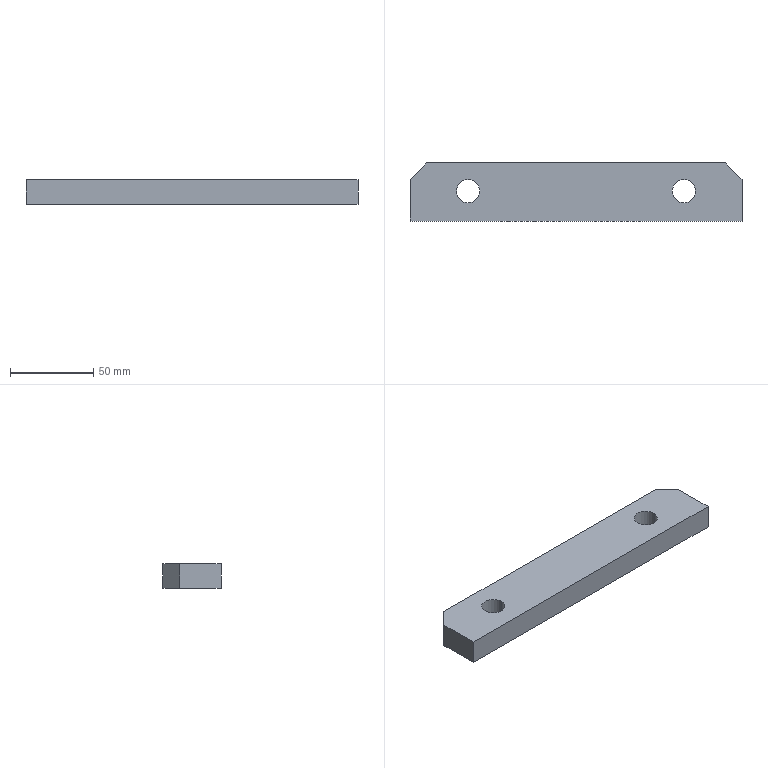Part | STEP file | Input 78 | 1 solid | 12 faces | box 200 x 35 x 15 mm | volume 98882 mm3 | plane 8 | cylinder 4 | commonest cylinder face diameters 14 x4
STEP:
#1=CARTESIAN_POINT('',(0.,0.,0.));
#2=DIRECTION('',(0.,0.,1.));
#3=DIRECTION('',(1.,0.,0.));
#4=AXIS2_PLACEMENT_3D('',#1,#2,#3);
#5=CARTESIAN_POINT('',(3960.,433.,-255.));
#6=VERTEX_POINT('',#5);
#7=CARTESIAN_POINT('',(3960.,433.,-270.));
#8=VERTEX_POINT('',#7);
#9=CARTESIAN_POINT('',(3960.,433.,-255.));
#10=DIRECTION('',(0.,0.,-1.));
#11=VECTOR('',#10,1.);
#12=LINE('',#9,#11);
#13=CARTESIAN_POINT('',(3967.,433.,-255.));
#14=DIRECTION('',(0.,0.,-1.));
#15=DIRECTION('',(-1.,0.,0.));
#16=AXIS2_PLACEMENT_3D('',#13,#14,#15);
#17=CYLINDRICAL_SURFACE('',#16,7.);
#18=CARTESIAN_POINT('',(6.283,0.));
#19=CARTESIAN_POINT('',(6.283,0.2273));
#20=CARTESIAN_POINT('',(6.283,0.6818));
#21=CARTESIAN_POINT('',(6.283,1.364));
#22=CARTESIAN_POINT('',(6.283,2.045));
#23=CARTESIAN_POINT('',(6.283,2.727));
#24=CARTESIAN_POINT('',(6.283,3.409));
#25=CARTESIAN_POINT('',(6.283,4.091));
#26=CARTESIAN_POINT('',(6.283,4.773));
#27=CARTESIAN_POINT('',(6.283,5.455));
#28=CARTESIAN_POINT('',(6.283,6.136));
#29=CARTESIAN_POINT('',(6.283,6.818));
#30=CARTESIAN_POINT('',(6.283,7.5));
#31=CARTESIAN_POINT('',(6.283,8.182));
#32=CARTESIAN_POINT('',(6.283,8.864));
#33=CARTESIAN_POINT('',(6.283,9.545));
#34=CARTESIAN_POINT('',(6.283,10.227));
#35=CARTESIAN_POINT('',(6.283,10.909));
#36=CARTESIAN_POINT('',(6.283,11.591));
#37=CARTESIAN_POINT('',(6.283,12.273));
#38=CARTESIAN_POINT('',(6.283,12.955));
#39=CARTESIAN_POINT('',(6.283,13.636));
#40=CARTESIAN_POINT('',(6.283,14.318));
#41=CARTESIAN_POINT('',(6.283,14.773));
#42=CARTESIAN_POINT('',(6.283,15.));
#43=B_SPLINE_CURVE_WITH_KNOTS('',3,(#18,#19,#20,#21,#22,#23,#24,#25,#26,#27,#28,#29,#30,#31,#32,#33,#34,#35,#36,#37,#38,#39,#40,#41,#42),.UNSPECIFIED.,.F.,.F.,(4,1,1,1,1,1,1,1,1,1,1,1,1,1,1,1,1,1,1,1,1,1,4),(0.,0.6818,1.364,2.045,2.727,3.409,4.091,4.773,5.455,6.136,6.818,7.5,8.182,8.864,9.545,10.227,10.909,11.591,12.273,12.955,13.636,14.318,15.),.QUASI_UNIFORM_KNOTS.);
#44=(GEOMETRIC_REPRESENTATION_CONTEXT(2)PARAMETRIC_REPRESENTATION_CONTEXT()REPRESENTATION_CONTEXT('',''));
#45=DEFINITIONAL_REPRESENTATION('',(#43),#44);
#46=PCURVE('',#17,#45);
#47=CARTESIAN_POINT('',(3967.,433.,-255.));
#48=DIRECTION('',(0.,0.,-1.));
#49=DIRECTION('',(-1.,0.,0.));
#50=AXIS2_PLACEMENT_3D('',#47,#48,#49);
#51=CYLINDRICAL_SURFACE('',#50,7.);
#52=CARTESIAN_POINT('',(0.,0.));
#53=DIRECTION('',(0.,1.));
#54=VECTOR('',#53,1.);
#55=LINE('',#52,#54);
#56=(GEOMETRIC_REPRESENTATION_CONTEXT(2)PARAMETRIC_REPRESENTATION_CONTEXT()REPRESENTATION_CONTEXT('',''));
#57=DEFINITIONAL_REPRESENTATION('',(#55),#56);
#58=PCURVE('',#51,#57);
#59=SURFACE_CURVE('',#12,(#46,#58),.PCURVE_S1.);
#60=EDGE_CURVE('',#6,#8,#59,.T.);
#61=ORIENTED_EDGE('',*,*,#60,.T.);
#62=CARTESIAN_POINT('',(3974.,433.,-270.));
#63=VERTEX_POINT('',#62);
#64=CARTESIAN_POINT('',(3967.,433.,-270.));
#65=DIRECTION('',(0.,0.,-1.));
#66=DIRECTION('',(-1.,0.,0.));
#67=AXIS2_PLACEMENT_3D('',#64,#65,#66);
#68=CIRCLE('',#67,7.);
#69=CARTESIAN_POINT('',(0.,15.));
#70=DIRECTION('',(1.,0.));
#71=VECTOR('',#70,1.);
#72=LINE('',#69,#71);
#73=(GEOMETRIC_REPRESENTATION_CONTEXT(2)PARAMETRIC_REPRESENTATION_CONTEXT()REPRESENTATION_CONTEXT('',''));
#74=DEFINITIONAL_REPRESENTATION('',(#72),#73);
#75=PCURVE('',#17,#74);
#76=CARTESIAN_POINT('',(4132.,450.,-270.));
#77=DIRECTION('',(0.,0.,1.));
#78=DIRECTION('',(1.,0.,0.));
#79=AXIS2_PLACEMENT_3D('',#76,#77,#78);
#80=PLANE('',#79);
#81=CARTESIAN_POINT('',(-172.,-17.));
#82=CARTESIAN_POINT('',(-172.,-4.876));
#83=CARTESIAN_POINT('',(-161.5,-10.938));
#84=CARTESIAN_POINT('',(-151.,-17.));
#85=CARTESIAN_POINT('',(-161.5,-23.062));
#86=CARTESIAN_POINT('',(-172.,-29.124));
#87=CARTESIAN_POINT('',(-172.,-17.));
#88=(BOUNDED_CURVE()B_SPLINE_CURVE(2,(#81,#82,#83,#84,#85,#86,#87),.UNSPECIFIED.,.T.,.F.)B_SPLINE_CURVE_WITH_KNOTS((1,2,2,2,2,1),(-2.094,0.,2.094,4.189,6.283,8.378),.UNSPECIFIED.)CURVE()GEOMETRIC_REPRESENTATION_ITEM()RATIONAL_B_SPLINE_CURVE((1.,0.5,1.,0.5,1.,0.5,1.))REPRESENTATION_ITEM(''));
#89=(GEOMETRIC_REPRESENTATION_CONTEXT(2)PARAMETRIC_REPRESENTATION_CONTEXT()REPRESENTATION_CONTEXT('',''));
#90=DEFINITIONAL_REPRESENTATION('',(#88),#89);
#91=PCURVE('',#80,#90);
#92=SURFACE_CURVE('',#68,(#75,#91),.PCURVE_S1.);
#93=EDGE_CURVE('',#63,#8,#92,.T.);
#94=ORIENTED_EDGE('',*,*,#93,.F.);
#95=CARTESIAN_POINT('',(3974.,433.,-255.));
#96=VERTEX_POINT('',#95);
#97=CARTESIAN_POINT('',(3974.,433.,-255.));
#98=DIRECTION('',(0.,0.,-1.));
#99=VECTOR('',#98,1.);
#100=LINE('',#97,#99);
#101=CARTESIAN_POINT('',(3.142,0.));
#102=DIRECTION('',(0.,1.));
#103=VECTOR('',#102,1.);
#104=LINE('',#101,#103);
#105=(GEOMETRIC_REPRESENTATION_CONTEXT(2)PARAMETRIC_REPRESENTATION_CONTEXT()REPRESENTATION_CONTEXT('',''));
#106=DEFINITIONAL_REPRESENTATION('',(#104),#105);
#107=PCURVE('',#17,#106);
#108=CARTESIAN_POINT('',(3.142,0.));
#109=DIRECTION('',(0.,1.));
#110=VECTOR('',#109,1.);
#111=LINE('',#108,#110);
#112=(GEOMETRIC_REPRESENTATION_CONTEXT(2)PARAMETRIC_REPRESENTATION_CONTEXT()REPRESENTATION_CONTEXT('',''));
#113=DEFINITIONAL_REPRESENTATION('',(#111),#112);
#114=PCURVE('',#51,#113);
#115=SURFACE_CURVE('',#100,(#107,#114),.PCURVE_S1.);
#116=EDGE_CURVE('',#96,#63,#115,.T.);
#117=ORIENTED_EDGE('',*,*,#116,.F.);
#118=CARTESIAN_POINT('',(3967.,433.,-255.));
#119=DIRECTION('',(0.,0.,-1.));
#120=DIRECTION('',(-1.,0.,0.));
#121=AXIS2_PLACEMENT_3D('',#118,#119,#120);
#122=CIRCLE('',#121,7.);
#123=CARTESIAN_POINT('',(0.,0.));
#124=DIRECTION('',(1.,0.));
#125=VECTOR('',#124,1.);
#126=LINE('',#123,#125);
#127=(GEOMETRIC_REPRESENTATION_CONTEXT(2)PARAMETRIC_REPRESENTATION_CONTEXT()REPRESENTATION_CONTEXT('',''));
#128=DEFINITIONAL_REPRESENTATION('',(#126),#127);
#129=PCURVE('',#17,#128);
#130=CARTESIAN_POINT('',(4132.,450.,-255.));
#131=DIRECTION('',(0.,0.,1.));
#132=DIRECTION('',(1.,0.,0.));
#133=AXIS2_PLACEMENT_3D('',#130,#131,#132);
#134=PLANE('',#133);
#135=CARTESIAN_POINT('',(-172.,-17.));
#136=CARTESIAN_POINT('',(-172.,-4.876));
#137=CARTESIAN_POINT('',(-161.5,-10.938));
#138=CARTESIAN_POINT('',(-151.,-17.));
#139=CARTESIAN_POINT('',(-161.5,-23.062));
#140=CARTESIAN_POINT('',(-172.,-29.124));
#141=CARTESIAN_POINT('',(-172.,-17.));
#142=(BOUNDED_CURVE()B_SPLINE_CURVE(2,(#135,#136,#137,#138,#139,#140,#141),.UNSPECIFIED.,.T.,.F.)B_SPLINE_CURVE_WITH_KNOTS((1,2,2,2,2,1),(-2.094,0.,2.094,4.189,6.283,8.378),.UNSPECIFIED.)CURVE()GEOMETRIC_REPRESENTATION_ITEM()RATIONAL_B_SPLINE_CURVE((1.,0.5,1.,0.5,1.,0.5,1.))REPRESENTATION_ITEM(''));
#143=(GEOMETRIC_REPRESENTATION_CONTEXT(2)PARAMETRIC_REPRESENTATION_CONTEXT()REPRESENTATION_CONTEXT('',''));
#144=DEFINITIONAL_REPRESENTATION('',(#142),#143);
#145=PCURVE('',#134,#144);
#146=SURFACE_CURVE('',#122,(#129,#145),.PCURVE_S1.);
#147=EDGE_CURVE('',#96,#6,#146,.T.);
#148=ORIENTED_EDGE('',*,*,#147,.T.);
#149=EDGE_LOOP('',(#61,#94,#117,#148));
#150=FACE_BOUND('',#149,.F.);
#151=ADVANCED_FACE('',(#150),#17,.F.);
#152=CARTESIAN_POINT('',(4090.,433.,-255.));
#153=VERTEX_POINT('',#152);
#154=CARTESIAN_POINT('',(4090.,433.,-270.));
#155=VERTEX_POINT('',#154);
#156=CARTESIAN_POINT('',(4090.,433.,-255.));
#157=DIRECTION('',(0.,0.,-1.));
#158=VECTOR('',#157,1.);
#159=LINE('',#156,#158);
#160=CARTESIAN_POINT('',(4097.,433.,-255.));
#161=DIRECTION('',(0.,0.,-1.));
#162=DIRECTION('',(-1.,0.,0.));
#163=AXIS2_PLACEMENT_3D('',#160,#161,#162);
#164=CYLINDRICAL_SURFACE('',#163,7.);
#165=CARTESIAN_POINT('',(6.283,0.));
#166=CARTESIAN_POINT('',(6.283,0.2273));
#167=CARTESIAN_POINT('',(6.283,0.6818));
#168=CARTESIAN_POINT('',(6.283,1.364));
#169=CARTESIAN_POINT('',(6.283,2.045));
#170=CARTESIAN_POINT('',(6.283,2.727));
#171=CARTESIAN_POINT('',(6.283,3.409));
#172=CARTESIAN_POINT('',(6.283,4.091));
#173=CARTESIAN_POINT('',(6.283,4.773));
#174=CARTESIAN_POINT('',(6.283,5.455));
#175=CARTESIAN_POINT('',(6.283,6.136));
#176=CARTESIAN_POINT('',(6.283,6.818));
#177=CARTESIAN_POINT('',(6.283,7.5));
#178=CARTESIAN_POINT('',(6.283,8.182));
#179=CARTESIAN_POINT('',(6.283,8.864));
#180=CARTESIAN_POINT('',(6.283,9.545));
#181=CARTESIAN_POINT('',(6.283,10.227));
#182=CARTESIAN_POINT('',(6.283,10.909));
#183=CARTESIAN_POINT('',(6.283,11.591));
#184=CARTESIAN_POINT('',(6.283,12.273));
#185=CARTESIAN_POINT('',(6.283,12.955));
#186=CARTESIAN_POINT('',(6.283,13.636));
#187=CARTESIAN_POINT('',(6.283,14.318));
#188=CARTESIAN_POINT('',(6.283,14.773));
#189=CARTESIAN_POINT('',(6.283,15.));
#190=B_SPLINE_CURVE_WITH_KNOTS('',3,(#165,#166,#167,#168,#169,#170,#171,#172,#173,#174,#175,#176,#177,#178,#179,#180,#181,#182,#183,#184,#185,#186,#187,#188,#189),.UNSPECIFIED.,.F.,.F.,(4,1,1,1,1,1,1,1,1,1,1,1,1,1,1,1,1,1,1,1,1,1,4),(0.,0.6818,1.364,2.045,2.727,3.409,4.091,4.773,5.455,6.136,6.818,7.5,8.182,8.864,9.545,10.227,10.909,11.591,12.273,12.955,13.636,14.318,15.),.QUASI_UNIFORM_KNOTS.);
#191=(GEOMETRIC_REPRESENTATION_CONTEXT(2)PARAMETRIC_REPRESENTATION_CONTEXT()REPRESENTATION_CONTEXT('',''));
#192=DEFINITIONAL_REPRESENTATION('',(#190),#191);
#193=PCURVE('',#164,#192);
#194=CARTESIAN_POINT('',(4097.,433.,-255.));
#195=DIRECTION('',(0.,0.,-1.));
#196=DIRECTION('',(-1.,0.,0.));
#197=AXIS2_PLACEMENT_3D('',#194,#195,#196);
#198=CYLINDRICAL_SURFACE('',#197,7.);
#199=CARTESIAN_POINT('',(0.,0.));
#200=DIRECTION('',(0.,1.));
#201=VECTOR('',#200,1.);
#202=LINE('',#199,#201);
#203=(GEOMETRIC_REPRESENTATION_CONTEXT(2)PARAMETRIC_REPRESENTATION_CONTEXT()REPRESENTATION_CONTEXT('',''));
#204=DEFINITIONAL_REPRESENTATION('',(#202),#203);
#205=PCURVE('',#198,#204);
#206=SURFACE_CURVE('',#159,(#193,#205),.PCURVE_S1.);
#207=EDGE_CURVE('',#153,#155,#206,.T.);
#208=ORIENTED_EDGE('',*,*,#207,.T.);
#209=CARTESIAN_POINT('',(4104.,433.,-270.));
#210=VERTEX_POINT('',#209);
#211=CARTESIAN_POINT('',(4097.,433.,-270.));
#212=DIRECTION('',(0.,0.,-1.));
#213=DIRECTION('',(-1.,0.,0.));
#214=AXIS2_PLACEMENT_3D('',#211,#212,#213);
#215=CIRCLE('',#214,7.);
#216=CARTESIAN_POINT('',(0.,15.));
#217=DIRECTION('',(1.,0.));
#218=VECTOR('',#217,1.);
#219=LINE('',#216,#218);
#220=(GEOMETRIC_REPRESENTATION_CONTEXT(2)PARAMETRIC_REPRESENTATION_CONTEXT()REPRESENTATION_CONTEXT('',''));
#221=DEFINITIONAL_REPRESENTATION('',(#219),#220);
#222=PCURVE('',#164,#221);
#223=CARTESIAN_POINT('',(-42.,-17.));
#224=CARTESIAN_POINT('',(-42.,-4.876));
#225=CARTESIAN_POINT('',(-31.5,-10.938));
#226=CARTESIAN_POINT('',(-21.,-17.));
#227=CARTESIAN_POINT('',(-31.5,-23.062));
#228=CARTESIAN_POINT('',(-42.,-29.124));
#229=CARTESIAN_POINT('',(-42.,-17.));
#230=(BOUNDED_CURVE()B_SPLINE_CURVE(2,(#223,#224,#225,#226,#227,#228,#229),.UNSPECIFIED.,.T.,.F.)B_SPLINE_CURVE_WITH_KNOTS((1,2,2,2,2,1),(-2.094,0.,2.094,4.189,6.283,8.378),.UNSPECIFIED.)CURVE()GEOMETRIC_REPRESENTATION_ITEM()RATIONAL_B_SPLINE_CURVE((1.,0.5,1.,0.5,1.,0.5,1.))REPRESENTATION_ITEM(''));
#231=(GEOMETRIC_REPRESENTATION_CONTEXT(2)PARAMETRIC_REPRESENTATION_CONTEXT()REPRESENTATION_CONTEXT('',''));
#232=DEFINITIONAL_REPRESENTATION('',(#230),#231);
#233=PCURVE('',#80,#232);
#234=SURFACE_CURVE('',#215,(#222,#233),.PCURVE_S1.);
#235=EDGE_CURVE('',#210,#155,#234,.T.);
#236=ORIENTED_EDGE('',*,*,#235,.F.);
#237=CARTESIAN_POINT('',(4104.,433.,-255.));
#238=VERTEX_POINT('',#237);
#239=CARTESIAN_POINT('',(4104.,433.,-255.));
#240=DIRECTION('',(0.,0.,-1.));
#241=VECTOR('',#240,1.);
#242=LINE('',#239,#241);
#243=CARTESIAN_POINT('',(3.142,0.));
#244=DIRECTION('',(0.,1.));
#245=VECTOR('',#244,1.);
#246=LINE('',#243,#245);
#247=(GEOMETRIC_REPRESENTATION_CONTEXT(2)PARAMETRIC_REPRESENTATION_CONTEXT()REPRESENTATION_CONTEXT('',''));
#248=DEFINITIONAL_REPRESENTATION('',(#246),#247);
#249=PCURVE('',#164,#248);
#250=CARTESIAN_POINT('',(3.142,0.));
#251=DIRECTION('',(0.,1.));
#252=VECTOR('',#251,1.);
#253=LINE('',#250,#252);
#254=(GEOMETRIC_REPRESENTATION_CONTEXT(2)PARAMETRIC_REPRESENTATION_CONTEXT()REPRESENTATION_CONTEXT('',''));
#255=DEFINITIONAL_REPRESENTATION('',(#253),#254);
#256=PCURVE('',#198,#255);
#257=SURFACE_CURVE('',#242,(#249,#256),.PCURVE_S1.);
#258=EDGE_CURVE('',#238,#210,#257,.T.);
#259=ORIENTED_EDGE('',*,*,#258,.F.);
#260=CARTESIAN_POINT('',(4097.,433.,-255.));
#261=DIRECTION('',(0.,0.,-1.));
#262=DIRECTION('',(-1.,0.,0.));
#263=AXIS2_PLACEMENT_3D('',#260,#261,#262);
#264=CIRCLE('',#263,7.);
#265=CARTESIAN_POINT('',(0.,0.));
#266=DIRECTION('',(1.,0.));
#267=VECTOR('',#266,1.);
#268=LINE('',#265,#267);
#269=(GEOMETRIC_REPRESENTATION_CONTEXT(2)PARAMETRIC_REPRESENTATION_CONTEXT()REPRESENTATION_CONTEXT('',''));
#270=DEFINITIONAL_REPRESENTATION('',(#268),#269);
#271=PCURVE('',#164,#270);
#272=CARTESIAN_POINT('',(-42.,-17.));
#273=CARTESIAN_POINT('',(-42.,-4.876));
#274=CARTESIAN_POINT('',(-31.5,-10.938));
#275=CARTESIAN_POINT('',(-21.,-17.));
#276=CARTESIAN_POINT('',(-31.5,-23.062));
#277=CARTESIAN_POINT('',(-42.,-29.124));
#278=CARTESIAN_POINT('',(-42.,-17.));
#279=(BOUNDED_CURVE()B_SPLINE_CURVE(2,(#272,#273,#274,#275,#276,#277,#278),.UNSPECIFIED.,.T.,.F.)B_SPLINE_CURVE_WITH_KNOTS((1,2,2,2,2,1),(-2.094,0.,2.094,4.189,6.283,8.378),.UNSPECIFIED.)CURVE()GEOMETRIC_REPRESENTATION_ITEM()RATIONAL_B_SPLINE_CURVE((1.,0.5,1.,0.5,1.,0.5,1.))REPRESENTATION_ITEM(''));
#280=(GEOMETRIC_REPRESENTATION_CONTEXT(2)PARAMETRIC_REPRESENTATION_CONTEXT()REPRESENTATION_CONTEXT('',''));
#281=DEFINITIONAL_REPRESENTATION('',(#279),#280);
#282=PCURVE('',#134,#281);
#283=SURFACE_CURVE('',#264,(#271,#282),.PCURVE_S1.);
#284=EDGE_CURVE('',#238,#153,#283,.T.);
#285=ORIENTED_EDGE('',*,*,#284,.T.);
#286=EDGE_LOOP('',(#208,#236,#259,#285));
#287=FACE_BOUND('',#286,.F.);
#288=ADVANCED_FACE('',(#287),#164,.F.);
#289=CARTESIAN_POINT('',(4132.,440.,-270.));
#290=VERTEX_POINT('',#289);
#291=CARTESIAN_POINT('',(4132.,415.,-270.));
#292=VERTEX_POINT('',#291);
#293=CARTESIAN_POINT('',(4132.,415.,-270.));
#294=DIRECTION('',(0.,-1.,0.));
#295=VECTOR('',#294,1.);
#296=LINE('',#293,#295);
#297=CARTESIAN_POINT('',(4132.,415.,-255.));
#298=DIRECTION('',(1.,0.,0.));
#299=DIRECTION('',(0.,0.,-1.));
#300=AXIS2_PLACEMENT_3D('',#297,#298,#299);
#301=PLANE('',#300);
#302=CARTESIAN_POINT('',(15.,0.));
#303=DIRECTION('',(0.,-1.));
#304=VECTOR('',#303,1.);
#305=LINE('',#302,#304);
#306=(GEOMETRIC_REPRESENTATION_CONTEXT(2)PARAMETRIC_REPRESENTATION_CONTEXT()REPRESENTATION_CONTEXT('',''));
#307=DEFINITIONAL_REPRESENTATION('',(#305),#306);
#308=PCURVE('',#301,#307);
#309=CARTESIAN_POINT('',(0.,-35.));
#310=DIRECTION('',(0.,-1.));
#311=VECTOR('',#310,1.);
#312=LINE('',#309,#311);
#313=(GEOMETRIC_REPRESENTATION_CONTEXT(2)PARAMETRIC_REPRESENTATION_CONTEXT()REPRESENTATION_CONTEXT('',''));
#314=DEFINITIONAL_REPRESENTATION('',(#312),#313);
#315=PCURVE('',#80,#314);
#316=SURFACE_CURVE('',#296,(#308,#315),.PCURVE_S1.);
#317=EDGE_CURVE('',#290,#292,#316,.T.);
#318=ORIENTED_EDGE('',*,*,#317,.F.);
#319=CARTESIAN_POINT('',(4132.,440.,-255.));
#320=VERTEX_POINT('',#319);
#321=CARTESIAN_POINT('',(4132.,440.,-255.));
#322=DIRECTION('',(0.,0.,-1.));
#323=VECTOR('',#322,1.);
#324=LINE('',#321,#323);
#325=CARTESIAN_POINT('',(0.,25.));
#326=DIRECTION('',(1.,0.));
#327=VECTOR('',#326,1.);
#328=LINE('',#325,#327);
#329=(GEOMETRIC_REPRESENTATION_CONTEXT(2)PARAMETRIC_REPRESENTATION_CONTEXT()REPRESENTATION_CONTEXT('',''));
#330=DEFINITIONAL_REPRESENTATION('',(#328),#329);
#331=PCURVE('',#301,#330);
#332=CARTESIAN_POINT('',(4132.,440.,-255.));
#333=DIRECTION('',(0.7071,0.7071,0.));
#334=DIRECTION('',(0.7071,-0.7071,0.));
#335=AXIS2_PLACEMENT_3D('',#332,#333,#334);
#336=PLANE('',#335);
#337=CARTESIAN_POINT('',(0.,0.));
#338=DIRECTION('',(0.,1.));
#339=VECTOR('',#338,1.);
#340=LINE('',#337,#339);
#341=(GEOMETRIC_REPRESENTATION_CONTEXT(2)PARAMETRIC_REPRESENTATION_CONTEXT()REPRESENTATION_CONTEXT('',''));
#342=DEFINITIONAL_REPRESENTATION('',(#340),#341);
#343=PCURVE('',#336,#342);
#344=SURFACE_CURVE('',#324,(#331,#343),.PCURVE_S1.);
#345=EDGE_CURVE('',#320,#290,#344,.T.);
#346=ORIENTED_EDGE('',*,*,#345,.F.);
#347=CARTESIAN_POINT('',(4132.,415.,-255.));
#348=VERTEX_POINT('',#347);
#349=CARTESIAN_POINT('',(4132.,415.,-255.));
#350=DIRECTION('',(0.,-1.,0.));
#351=VECTOR('',#350,1.);
#352=LINE('',#349,#351);
#353=CARTESIAN_POINT('',(0.,0.));
#354=DIRECTION('',(0.,-1.));
#355=VECTOR('',#354,1.);
#356=LINE('',#353,#355);
#357=(GEOMETRIC_REPRESENTATION_CONTEXT(2)PARAMETRIC_REPRESENTATION_CONTEXT()REPRESENTATION_CONTEXT('',''));
#358=DEFINITIONAL_REPRESENTATION('',(#356),#357);
#359=PCURVE('',#301,#358);
#360=CARTESIAN_POINT('',(0.,-35.));
#361=DIRECTION('',(0.,-1.));
#362=VECTOR('',#361,1.);
#363=LINE('',#360,#362);
#364=(GEOMETRIC_REPRESENTATION_CONTEXT(2)PARAMETRIC_REPRESENTATION_CONTEXT()REPRESENTATION_CONTEXT('',''));
#365=DEFINITIONAL_REPRESENTATION('',(#363),#364);
#366=PCURVE('',#134,#365);
#367=SURFACE_CURVE('',#352,(#359,#366),.PCURVE_S1.);
#368=EDGE_CURVE('',#320,#348,#367,.T.);
#369=ORIENTED_EDGE('',*,*,#368,.T.);
#370=CARTESIAN_POINT('',(4132.,415.,-255.));
#371=DIRECTION('',(0.,0.,-1.));
#372=VECTOR('',#371,1.);
#373=LINE('',#370,#372);
#374=CARTESIAN_POINT('',(0.,0.));
#375=DIRECTION('',(1.,0.));
#376=VECTOR('',#375,1.);
#377=LINE('',#374,#376);
#378=(GEOMETRIC_REPRESENTATION_CONTEXT(2)PARAMETRIC_REPRESENTATION_CONTEXT()REPRESENTATION_CONTEXT('',''));
#379=DEFINITIONAL_REPRESENTATION('',(#377),#378);
#380=PCURVE('',#301,#379);
#381=CARTESIAN_POINT('',(4132.,415.,-255.));
#382=DIRECTION('',(0.,-1.,0.));
#383=DIRECTION('',(0.,0.,1.));
#384=AXIS2_PLACEMENT_3D('',#381,#382,#383);
#385=PLANE('',#384);
#386=CARTESIAN_POINT('',(0.,0.));
#387=DIRECTION('',(-1.,0.));
#388=VECTOR('',#387,1.);
#389=LINE('',#386,#388);
#390=(GEOMETRIC_REPRESENTATION_CONTEXT(2)PARAMETRIC_REPRESENTATION_CONTEXT()REPRESENTATION_CONTEXT('',''));
#391=DEFINITIONAL_REPRESENTATION('',(#389),#390);
#392=PCURVE('',#385,#391);
#393=SURFACE_CURVE('',#373,(#380,#392),.PCURVE_S1.);
#394=EDGE_CURVE('',#348,#292,#393,.T.);
#395=ORIENTED_EDGE('',*,*,#394,.T.);
#396=EDGE_LOOP('',(#318,#346,#369,#395));
#397=FACE_BOUND('',#396,.T.);
#398=ADVANCED_FACE('',(#397),#301,.T.);
#399=CARTESIAN_POINT('',(4122.,450.,-270.));
#400=VERTEX_POINT('',#399);
#401=CARTESIAN_POINT('',(4132.,440.,-270.));
#402=DIRECTION('',(0.7071,-0.7071,0.));
#403=VECTOR('',#402,1.);
#404=LINE('',#401,#403);
#405=CARTESIAN_POINT('',(0.,15.));
#406=DIRECTION('',(1.,0.));
#407=VECTOR('',#406,1.);
#408=LINE('',#405,#407);
#409=(GEOMETRIC_REPRESENTATION_CONTEXT(2)PARAMETRIC_REPRESENTATION_CONTEXT()REPRESENTATION_CONTEXT('',''));
#410=DEFINITIONAL_REPRESENTATION('',(#408),#409);
#411=PCURVE('',#336,#410);
#412=CARTESIAN_POINT('',(0.,-10.));
#413=DIRECTION('',(0.7071,-0.7071));
#414=VECTOR('',#413,1.);
#415=LINE('',#412,#414);
#416=(GEOMETRIC_REPRESENTATION_CONTEXT(2)PARAMETRIC_REPRESENTATION_CONTEXT()REPRESENTATION_CONTEXT('',''));
#417=DEFINITIONAL_REPRESENTATION('',(#415),#416);
#418=PCURVE('',#80,#417);
#419=SURFACE_CURVE('',#404,(#411,#418),.PCURVE_S1.);
#420=EDGE_CURVE('',#400,#290,#419,.T.);
#421=ORIENTED_EDGE('',*,*,#420,.F.);
#422=CARTESIAN_POINT('',(4122.,450.,-255.));
#423=VERTEX_POINT('',#422);
#424=CARTESIAN_POINT('',(4122.,450.,-255.));
#425=DIRECTION('',(0.,0.,-1.));
#426=VECTOR('',#425,1.);
#427=LINE('',#424,#426);
#428=CARTESIAN_POINT('',(-14.142,0.));
#429=DIRECTION('',(0.,1.));
#430=VECTOR('',#429,1.);
#431=LINE('',#428,#430);
#432=(GEOMETRIC_REPRESENTATION_CONTEXT(2)PARAMETRIC_REPRESENTATION_CONTEXT()REPRESENTATION_CONTEXT('',''));
#433=DEFINITIONAL_REPRESENTATION('',(#431),#432);
#434=PCURVE('',#336,#433);
#435=CARTESIAN_POINT('',(4122.,450.,-255.));
#436=DIRECTION('',(0.,1.,0.));
#437=DIRECTION('',(0.,0.,-1.));
#438=AXIS2_PLACEMENT_3D('',#435,#436,#437);
#439=PLANE('',#438);
#440=CARTESIAN_POINT('',(0.,0.));
#441=DIRECTION('',(1.,0.));
#442=VECTOR('',#441,1.);
#443=LINE('',#440,#442);
#444=(GEOMETRIC_REPRESENTATION_CONTEXT(2)PARAMETRIC_REPRESENTATION_CONTEXT()REPRESENTATION_CONTEXT('',''));
#445=DEFINITIONAL_REPRESENTATION('',(#443),#444);
#446=PCURVE('',#439,#445);
#447=SURFACE_CURVE('',#427,(#434,#446),.PCURVE_S1.);
#448=EDGE_CURVE('',#423,#400,#447,.T.);
#449=ORIENTED_EDGE('',*,*,#448,.F.);
#450=CARTESIAN_POINT('',(4132.,440.,-255.));
#451=DIRECTION('',(0.7071,-0.7071,0.));
#452=VECTOR('',#451,1.);
#453=LINE('',#450,#452);
#454=CARTESIAN_POINT('',(0.,0.));
#455=DIRECTION('',(1.,0.));
#456=VECTOR('',#455,1.);
#457=LINE('',#454,#456);
#458=(GEOMETRIC_REPRESENTATION_CONTEXT(2)PARAMETRIC_REPRESENTATION_CONTEXT()REPRESENTATION_CONTEXT('',''));
#459=DEFINITIONAL_REPRESENTATION('',(#457),#458);
#460=PCURVE('',#336,#459);
#461=CARTESIAN_POINT('',(0.,-10.));
#462=DIRECTION('',(0.7071,-0.7071));
#463=VECTOR('',#462,1.);
#464=LINE('',#461,#463);
#465=(GEOMETRIC_REPRESENTATION_CONTEXT(2)PARAMETRIC_REPRESENTATION_CONTEXT()REPRESENTATION_CONTEXT('',''));
#466=DEFINITIONAL_REPRESENTATION('',(#464),#465);
#467=PCURVE('',#134,#466);
#468=SURFACE_CURVE('',#453,(#460,#467),.PCURVE_S1.);
#469=EDGE_CURVE('',#423,#320,#468,.T.);
#470=ORIENTED_EDGE('',*,*,#469,.T.);
#471=ORIENTED_EDGE('',*,*,#345,.T.);
#472=EDGE_LOOP('',(#421,#449,#470,#471));
#473=FACE_BOUND('',#472,.T.);
#474=ADVANCED_FACE('',(#473),#336,.T.);
#475=CARTESIAN_POINT('',(3942.,450.,-270.));
#476=VERTEX_POINT('',#475);
#477=CARTESIAN_POINT('',(4122.,450.,-270.));
#478=DIRECTION('',(1.,0.,0.));
#479=VECTOR('',#478,1.);
#480=LINE('',#477,#479);
#481=CARTESIAN_POINT('',(15.,0.));
#482=DIRECTION('',(0.,-1.));
#483=VECTOR('',#482,1.);
#484=LINE('',#481,#483);
#485=(GEOMETRIC_REPRESENTATION_CONTEXT(2)PARAMETRIC_REPRESENTATION_CONTEXT()REPRESENTATION_CONTEXT('',''));
#486=DEFINITIONAL_REPRESENTATION('',(#484),#485);
#487=PCURVE('',#439,#486);
#488=CARTESIAN_POINT('',(-10.,0.));
#489=DIRECTION('',(1.,0.));
#490=VECTOR('',#489,1.);
#491=LINE('',#488,#490);
#492=(GEOMETRIC_REPRESENTATION_CONTEXT(2)PARAMETRIC_REPRESENTATION_CONTEXT()REPRESENTATION_CONTEXT('',''));
#493=DEFINITIONAL_REPRESENTATION('',(#491),#492);
#494=PCURVE('',#80,#493);
#495=SURFACE_CURVE('',#480,(#487,#494),.PCURVE_S1.);
#496=EDGE_CURVE('',#476,#400,#495,.T.);
#497=ORIENTED_EDGE('',*,*,#496,.F.);
#498=CARTESIAN_POINT('',(3942.,450.,-255.));
#499=VERTEX_POINT('',#498);
#500=CARTESIAN_POINT('',(3942.,450.,-255.));
#501=DIRECTION('',(0.,0.,-1.));
#502=VECTOR('',#501,1.);
#503=LINE('',#500,#502);
#504=CARTESIAN_POINT('',(0.,180.));
#505=DIRECTION('',(1.,0.));
#506=VECTOR('',#505,1.);
#507=LINE('',#504,#506);
#508=(GEOMETRIC_REPRESENTATION_CONTEXT(2)PARAMETRIC_REPRESENTATION_CONTEXT()REPRESENTATION_CONTEXT('',''));
#509=DEFINITIONAL_REPRESENTATION('',(#507),#508);
#510=PCURVE('',#439,#509);
#511=CARTESIAN_POINT('',(3942.,450.,-255.));
#512=DIRECTION('',(-0.7071,0.7071,0.));
#513=DIRECTION('',(0.7071,0.7071,0.));
#514=AXIS2_PLACEMENT_3D('',#511,#512,#513);
#515=PLANE('',#514);
#516=CARTESIAN_POINT('',(0.,0.));
#517=DIRECTION('',(0.,1.));
#518=VECTOR('',#517,1.);
#519=LINE('',#516,#518);
#520=(GEOMETRIC_REPRESENTATION_CONTEXT(2)PARAMETRIC_REPRESENTATION_CONTEXT()REPRESENTATION_CONTEXT('',''));
#521=DEFINITIONAL_REPRESENTATION('',(#519),#520);
#522=PCURVE('',#515,#521);
#523=SURFACE_CURVE('',#503,(#510,#522),.PCURVE_S1.);
#524=EDGE_CURVE('',#499,#476,#523,.T.);
#525=ORIENTED_EDGE('',*,*,#524,.F.);
#526=CARTESIAN_POINT('',(4122.,450.,-255.));
#527=DIRECTION('',(1.,0.,0.));
#528=VECTOR('',#527,1.);
#529=LINE('',#526,#528);
#530=CARTESIAN_POINT('',(0.,0.));
#531=DIRECTION('',(0.,-1.));
#532=VECTOR('',#531,1.);
#533=LINE('',#530,#532);
#534=(GEOMETRIC_REPRESENTATION_CONTEXT(2)PARAMETRIC_REPRESENTATION_CONTEXT()REPRESENTATION_CONTEXT('',''));
#535=DEFINITIONAL_REPRESENTATION('',(#533),#534);
#536=PCURVE('',#439,#535);
#537=CARTESIAN_POINT('',(-10.,0.));
#538=DIRECTION('',(1.,0.));
#539=VECTOR('',#538,1.);
#540=LINE('',#537,#539);
#541=(GEOMETRIC_REPRESENTATION_CONTEXT(2)PARAMETRIC_REPRESENTATION_CONTEXT()REPRESENTATION_CONTEXT('',''));
#542=DEFINITIONAL_REPRESENTATION('',(#540),#541);
#543=PCURVE('',#134,#542);
#544=SURFACE_CURVE('',#529,(#536,#543),.PCURVE_S1.);
#545=EDGE_CURVE('',#499,#423,#544,.T.);
#546=ORIENTED_EDGE('',*,*,#545,.T.);
#547=ORIENTED_EDGE('',*,*,#448,.T.);
#548=EDGE_LOOP('',(#497,#525,#546,#547));
#549=FACE_BOUND('',#548,.T.);
#550=ADVANCED_FACE('',(#549),#439,.T.);
#551=CARTESIAN_POINT('',(3932.,440.,-270.));
#552=VERTEX_POINT('',#551);
#553=CARTESIAN_POINT('',(3942.,450.,-270.));
#554=DIRECTION('',(0.7071,0.7071,0.));
#555=VECTOR('',#554,1.);
#556=LINE('',#553,#555);
#557=CARTESIAN_POINT('',(0.,15.));
#558=DIRECTION('',(1.,0.));
#559=VECTOR('',#558,1.);
#560=LINE('',#557,#559);
#561=(GEOMETRIC_REPRESENTATION_CONTEXT(2)PARAMETRIC_REPRESENTATION_CONTEXT()REPRESENTATION_CONTEXT('',''));
#562=DEFINITIONAL_REPRESENTATION('',(#560),#561);
#563=PCURVE('',#515,#562);
#564=CARTESIAN_POINT('',(-190.,0.));
#565=DIRECTION('',(0.7071,0.7071));
#566=VECTOR('',#565,1.);
#567=LINE('',#564,#566);
#568=(GEOMETRIC_REPRESENTATION_CONTEXT(2)PARAMETRIC_REPRESENTATION_CONTEXT()REPRESENTATION_CONTEXT('',''));
#569=DEFINITIONAL_REPRESENTATION('',(#567),#568);
#570=PCURVE('',#80,#569);
#571=SURFACE_CURVE('',#556,(#563,#570),.PCURVE_S1.);
#572=EDGE_CURVE('',#552,#476,#571,.T.);
#573=ORIENTED_EDGE('',*,*,#572,.F.);
#574=CARTESIAN_POINT('',(3932.,440.,-255.));
#575=VERTEX_POINT('',#574);
#576=CARTESIAN_POINT('',(3932.,440.,-255.));
#577=DIRECTION('',(0.,0.,-1.));
#578=VECTOR('',#577,1.);
#579=LINE('',#576,#578);
#580=CARTESIAN_POINT('',(-14.142,0.));
#581=DIRECTION('',(0.,1.));
#582=VECTOR('',#581,1.);
#583=LINE('',#580,#582);
#584=(GEOMETRIC_REPRESENTATION_CONTEXT(2)PARAMETRIC_REPRESENTATION_CONTEXT()REPRESENTATION_CONTEXT('',''));
#585=DEFINITIONAL_REPRESENTATION('',(#583),#584);
#586=PCURVE('',#515,#585);
#587=CARTESIAN_POINT('',(3932.,415.,-255.));
#588=DIRECTION('',(-1.,0.,0.));
#589=DIRECTION('',(0.,0.,1.));
#590=AXIS2_PLACEMENT_3D('',#587,#588,#589);
#591=PLANE('',#590);
#592=CARTESIAN_POINT('',(0.,25.));
#593=DIRECTION('',(-1.,0.));
#594=VECTOR('',#593,1.);
#595=LINE('',#592,#594);
#596=(GEOMETRIC_REPRESENTATION_CONTEXT(2)PARAMETRIC_REPRESENTATION_CONTEXT()REPRESENTATION_CONTEXT('',''));
#597=DEFINITIONAL_REPRESENTATION('',(#595),#596);
#598=PCURVE('',#591,#597);
#599=SURFACE_CURVE('',#579,(#586,#598),.PCURVE_S1.);
#600=EDGE_CURVE('',#575,#552,#599,.T.);
#601=ORIENTED_EDGE('',*,*,#600,.F.);
#602=CARTESIAN_POINT('',(3942.,450.,-255.));
#603=DIRECTION('',(0.7071,0.7071,0.));
#604=VECTOR('',#603,1.);
#605=LINE('',#602,#604);
#606=CARTESIAN_POINT('',(0.,0.));
#607=DIRECTION('',(1.,0.));
#608=VECTOR('',#607,1.);
#609=LINE('',#606,#608);
#610=(GEOMETRIC_REPRESENTATION_CONTEXT(2)PARAMETRIC_REPRESENTATION_CONTEXT()REPRESENTATION_CONTEXT('',''));
#611=DEFINITIONAL_REPRESENTATION('',(#609),#610);
#612=PCURVE('',#515,#611);
#613=CARTESIAN_POINT('',(-190.,0.));
#614=DIRECTION('',(0.7071,0.7071));
#615=VECTOR('',#614,1.);
#616=LINE('',#613,#615);
#617=(GEOMETRIC_REPRESENTATION_CONTEXT(2)PARAMETRIC_REPRESENTATION_CONTEXT()REPRESENTATION_CONTEXT('',''));
#618=DEFINITIONAL_REPRESENTATION('',(#616),#617);
#619=PCURVE('',#134,#618);
#620=SURFACE_CURVE('',#605,(#612,#619),.PCURVE_S1.);
#621=EDGE_CURVE('',#575,#499,#620,.T.);
#622=ORIENTED_EDGE('',*,*,#621,.T.);
#623=ORIENTED_EDGE('',*,*,#524,.T.);
#624=EDGE_LOOP('',(#573,#601,#622,#623));
#625=FACE_BOUND('',#624,.T.);
#626=ADVANCED_FACE('',(#625),#515,.T.);
#627=CARTESIAN_POINT('',(3932.,415.,-270.));
#628=VERTEX_POINT('',#627);
#629=CARTESIAN_POINT('',(3932.,415.,-270.));
#630=DIRECTION('',(0.,1.,0.));
#631=VECTOR('',#630,1.);
#632=LINE('',#629,#631);
#633=CARTESIAN_POINT('',(-15.,0.));
#634=DIRECTION('',(0.,1.));
#635=VECTOR('',#634,1.);
#636=LINE('',#633,#635);
#637=(GEOMETRIC_REPRESENTATION_CONTEXT(2)PARAMETRIC_REPRESENTATION_CONTEXT()REPRESENTATION_CONTEXT('',''));
#638=DEFINITIONAL_REPRESENTATION('',(#636),#637);
#639=PCURVE('',#591,#638);
#640=CARTESIAN_POINT('',(-200.,-35.));
#641=DIRECTION('',(0.,1.));
#642=VECTOR('',#641,1.);
#643=LINE('',#640,#642);
#644=(GEOMETRIC_REPRESENTATION_CONTEXT(2)PARAMETRIC_REPRESENTATION_CONTEXT()REPRESENTATION_CONTEXT('',''));
#645=DEFINITIONAL_REPRESENTATION('',(#643),#644);
#646=PCURVE('',#80,#645);
#647=SURFACE_CURVE('',#632,(#639,#646),.PCURVE_S1.);
#648=EDGE_CURVE('',#628,#552,#647,.T.);
#649=ORIENTED_EDGE('',*,*,#648,.F.);
#650=CARTESIAN_POINT('',(3932.,415.,-255.));
#651=VERTEX_POINT('',#650);
#652=CARTESIAN_POINT('',(3932.,415.,-255.));
#653=DIRECTION('',(0.,0.,-1.));
#654=VECTOR('',#653,1.);
#655=LINE('',#652,#654);
#656=CARTESIAN_POINT('',(0.,0.));
#657=DIRECTION('',(-1.,0.));
#658=VECTOR('',#657,1.);
#659=LINE('',#656,#658);
#660=(GEOMETRIC_REPRESENTATION_CONTEXT(2)PARAMETRIC_REPRESENTATION_CONTEXT()REPRESENTATION_CONTEXT('',''));
#661=DEFINITIONAL_REPRESENTATION('',(#659),#660);
#662=PCURVE('',#591,#661);
#663=CARTESIAN_POINT('',(0.,200.));
#664=DIRECTION('',(-1.,0.));
#665=VECTOR('',#664,1.);
#666=LINE('',#663,#665);
#667=(GEOMETRIC_REPRESENTATION_CONTEXT(2)PARAMETRIC_REPRESENTATION_CONTEXT()REPRESENTATION_CONTEXT('',''));
#668=DEFINITIONAL_REPRESENTATION('',(#666),#667);
#669=PCURVE('',#385,#668);
#670=SURFACE_CURVE('',#655,(#662,#669),.PCURVE_S1.);
#671=EDGE_CURVE('',#651,#628,#670,.T.);
#672=ORIENTED_EDGE('',*,*,#671,.F.);
#673=CARTESIAN_POINT('',(3932.,415.,-255.));
#674=DIRECTION('',(0.,1.,0.));
#675=VECTOR('',#674,1.);
#676=LINE('',#673,#675);
#677=CARTESIAN_POINT('',(0.,0.));
#678=DIRECTION('',(0.,1.));
#679=VECTOR('',#678,1.);
#680=LINE('',#677,#679);
#681=(GEOMETRIC_REPRESENTATION_CONTEXT(2)PARAMETRIC_REPRESENTATION_CONTEXT()REPRESENTATION_CONTEXT('',''));
#682=DEFINITIONAL_REPRESENTATION('',(#680),#681);
#683=PCURVE('',#591,#682);
#684=CARTESIAN_POINT('',(-200.,-35.));
#685=DIRECTION('',(0.,1.));
#686=VECTOR('',#685,1.);
#687=LINE('',#684,#686);
#688=(GEOMETRIC_REPRESENTATION_CONTEXT(2)PARAMETRIC_REPRESENTATION_CONTEXT()REPRESENTATION_CONTEXT('',''));
#689=DEFINITIONAL_REPRESENTATION('',(#687),#688);
#690=PCURVE('',#134,#689);
#691=SURFACE_CURVE('',#676,(#683,#690),.PCURVE_S1.);
#692=EDGE_CURVE('',#651,#575,#691,.T.);
#693=ORIENTED_EDGE('',*,*,#692,.T.);
#694=ORIENTED_EDGE('',*,*,#600,.T.);
#695=EDGE_LOOP('',(#649,#672,#693,#694));
#696=FACE_BOUND('',#695,.T.);
#697=ADVANCED_FACE('',(#696),#591,.T.);
#698=CARTESIAN_POINT('',(4132.,415.,-270.));
#699=DIRECTION('',(-1.,0.,0.));
#700=VECTOR('',#699,1.);
#701=LINE('',#698,#700);
#702=CARTESIAN_POINT('',(-15.,0.));
#703=DIRECTION('',(0.,1.));
#704=VECTOR('',#703,1.);
#705=LINE('',#702,#704);
#706=(GEOMETRIC_REPRESENTATION_CONTEXT(2)PARAMETRIC_REPRESENTATION_CONTEXT()REPRESENTATION_CONTEXT('',''));
#707=DEFINITIONAL_REPRESENTATION('',(#705),#706);
#708=PCURVE('',#385,#707);
#709=CARTESIAN_POINT('',(0.,-35.));
#710=DIRECTION('',(-1.,0.));
#711=VECTOR('',#710,1.);
#712=LINE('',#709,#711);
#713=(GEOMETRIC_REPRESENTATION_CONTEXT(2)PARAMETRIC_REPRESENTATION_CONTEXT()REPRESENTATION_CONTEXT('',''));
#714=DEFINITIONAL_REPRESENTATION('',(#712),#713);
#715=PCURVE('',#80,#714);
#716=SURFACE_CURVE('',#701,(#708,#715),.PCURVE_S1.);
#717=EDGE_CURVE('',#292,#628,#716,.T.);
#718=ORIENTED_EDGE('',*,*,#717,.F.);
#719=ORIENTED_EDGE('',*,*,#394,.F.);
#720=CARTESIAN_POINT('',(4132.,415.,-255.));
#721=DIRECTION('',(-1.,0.,0.));
#722=VECTOR('',#721,1.);
#723=LINE('',#720,#722);
#724=CARTESIAN_POINT('',(0.,0.));
#725=DIRECTION('',(0.,1.));
#726=VECTOR('',#725,1.);
#727=LINE('',#724,#726);
#728=(GEOMETRIC_REPRESENTATION_CONTEXT(2)PARAMETRIC_REPRESENTATION_CONTEXT()REPRESENTATION_CONTEXT('',''));
#729=DEFINITIONAL_REPRESENTATION('',(#727),#728);
#730=PCURVE('',#385,#729);
#731=CARTESIAN_POINT('',(0.,-35.));
#732=DIRECTION('',(-1.,0.));
#733=VECTOR('',#732,1.);
#734=LINE('',#731,#733);
#735=(GEOMETRIC_REPRESENTATION_CONTEXT(2)PARAMETRIC_REPRESENTATION_CONTEXT()REPRESENTATION_CONTEXT('',''));
#736=DEFINITIONAL_REPRESENTATION('',(#734),#735);
#737=PCURVE('',#134,#736);
#738=SURFACE_CURVE('',#723,(#730,#737),.PCURVE_S1.);
#739=EDGE_CURVE('',#348,#651,#738,.T.);
#740=ORIENTED_EDGE('',*,*,#739,.T.);
#741=ORIENTED_EDGE('',*,*,#671,.T.);
#742=EDGE_LOOP('',(#718,#719,#740,#741));
#743=FACE_BOUND('',#742,.T.);
#744=ADVANCED_FACE('',(#743),#385,.T.);
#745=CARTESIAN_POINT('',(3967.,433.,-255.));
#746=DIRECTION('',(0.,0.,-1.));
#747=DIRECTION('',(-1.,0.,0.));
#748=AXIS2_PLACEMENT_3D('',#745,#746,#747);
#749=CIRCLE('',#748,7.);
#750=CARTESIAN_POINT('',(-172.,-17.));
#751=CARTESIAN_POINT('',(-172.,-4.876));
#752=CARTESIAN_POINT('',(-161.5,-10.938));
#753=CARTESIAN_POINT('',(-151.,-17.));
#754=CARTESIAN_POINT('',(-161.5,-23.062));
#755=CARTESIAN_POINT('',(-172.,-29.124));
#756=CARTESIAN_POINT('',(-172.,-17.));
#757=(BOUNDED_CURVE()B_SPLINE_CURVE(2,(#750,#751,#752,#753,#754,#755,#756),.UNSPECIFIED.,.T.,.F.)B_SPLINE_CURVE_WITH_KNOTS((1,2,2,2,2,1),(-2.094,0.,2.094,4.189,6.283,8.378),.UNSPECIFIED.)CURVE()GEOMETRIC_REPRESENTATION_ITEM()RATIONAL_B_SPLINE_CURVE((1.,0.5,1.,0.5,1.,0.5,1.))REPRESENTATION_ITEM(''));
#758=(GEOMETRIC_REPRESENTATION_CONTEXT(2)PARAMETRIC_REPRESENTATION_CONTEXT()REPRESENTATION_CONTEXT('',''));
#759=DEFINITIONAL_REPRESENTATION('',(#757),#758);
#760=PCURVE('',#134,#759);
#761=CARTESIAN_POINT('',(0.,0.));
#762=DIRECTION('',(1.,0.));
#763=VECTOR('',#762,1.);
#764=LINE('',#761,#763);
#765=(GEOMETRIC_REPRESENTATION_CONTEXT(2)PARAMETRIC_REPRESENTATION_CONTEXT()REPRESENTATION_CONTEXT('',''));
#766=DEFINITIONAL_REPRESENTATION('',(#764),#765);
#767=PCURVE('',#51,#766);
#768=SURFACE_CURVE('',#749,(#760,#767),.PCURVE_S1.);
#769=EDGE_CURVE('',#6,#96,#768,.T.);
#770=ORIENTED_EDGE('',*,*,#769,.T.);
#771=ORIENTED_EDGE('',*,*,#147,.T.);
#772=EDGE_LOOP('',(#770,#771));
#773=FACE_BOUND('',#772,.T.);
#774=CARTESIAN_POINT('',(4097.,433.,-255.));
#775=DIRECTION('',(0.,0.,-1.));
#776=DIRECTION('',(-1.,0.,0.));
#777=AXIS2_PLACEMENT_3D('',#774,#775,#776);
#778=CIRCLE('',#777,7.);
#779=CARTESIAN_POINT('',(-42.,-17.));
#780=CARTESIAN_POINT('',(-42.,-4.876));
#781=CARTESIAN_POINT('',(-31.5,-10.938));
#782=CARTESIAN_POINT('',(-21.,-17.));
#783=CARTESIAN_POINT('',(-31.5,-23.062));
#784=CARTESIAN_POINT('',(-42.,-29.124));
#785=CARTESIAN_POINT('',(-42.,-17.));
#786=(BOUNDED_CURVE()B_SPLINE_CURVE(2,(#779,#780,#781,#782,#783,#784,#785),.UNSPECIFIED.,.T.,.F.)B_SPLINE_CURVE_WITH_KNOTS((1,2,2,2,2,1),(-2.094,0.,2.094,4.189,6.283,8.378),.UNSPECIFIED.)CURVE()GEOMETRIC_REPRESENTATION_ITEM()RATIONAL_B_SPLINE_CURVE((1.,0.5,1.,0.5,1.,0.5,1.))REPRESENTATION_ITEM(''));
#787=(GEOMETRIC_REPRESENTATION_CONTEXT(2)PARAMETRIC_REPRESENTATION_CONTEXT()REPRESENTATION_CONTEXT('',''));
#788=DEFINITIONAL_REPRESENTATION('',(#786),#787);
#789=PCURVE('',#134,#788);
#790=CARTESIAN_POINT('',(0.,0.));
#791=DIRECTION('',(1.,0.));
#792=VECTOR('',#791,1.);
#793=LINE('',#790,#792);
#794=(GEOMETRIC_REPRESENTATION_CONTEXT(2)PARAMETRIC_REPRESENTATION_CONTEXT()REPRESENTATION_CONTEXT('',''));
#795=DEFINITIONAL_REPRESENTATION('',(#793),#794);
#796=PCURVE('',#198,#795);
#797=SURFACE_CURVE('',#778,(#789,#796),.PCURVE_S1.);
#798=EDGE_CURVE('',#153,#238,#797,.T.);
#799=ORIENTED_EDGE('',*,*,#798,.T.);
#800=ORIENTED_EDGE('',*,*,#284,.T.);
#801=EDGE_LOOP('',(#799,#800));
#802=FACE_BOUND('',#801,.T.);
#803=ORIENTED_EDGE('',*,*,#368,.F.);
#804=ORIENTED_EDGE('',*,*,#469,.F.);
#805=ORIENTED_EDGE('',*,*,#545,.F.);
#806=ORIENTED_EDGE('',*,*,#621,.F.);
#807=ORIENTED_EDGE('',*,*,#692,.F.);
#808=ORIENTED_EDGE('',*,*,#739,.F.);
#809=EDGE_LOOP('',(#803,#804,#805,#806,#807,#808));
#810=FACE_BOUND('',#809,.T.);
#811=ADVANCED_FACE('',(#773,#802,#810),#134,.T.);
#812=CARTESIAN_POINT('',(3967.,433.,-270.));
#813=DIRECTION('',(0.,0.,-1.));
#814=DIRECTION('',(-1.,0.,0.));
#815=AXIS2_PLACEMENT_3D('',#812,#813,#814);
#816=CIRCLE('',#815,7.);
#817=CARTESIAN_POINT('',(-172.,-17.));
#818=CARTESIAN_POINT('',(-172.,-4.876));
#819=CARTESIAN_POINT('',(-161.5,-10.938));
#820=CARTESIAN_POINT('',(-151.,-17.));
#821=CARTESIAN_POINT('',(-161.5,-23.062));
#822=CARTESIAN_POINT('',(-172.,-29.124));
#823=CARTESIAN_POINT('',(-172.,-17.));
#824=(BOUNDED_CURVE()B_SPLINE_CURVE(2,(#817,#818,#819,#820,#821,#822,#823),.UNSPECIFIED.,.T.,.F.)B_SPLINE_CURVE_WITH_KNOTS((1,2,2,2,2,1),(-2.094,0.,2.094,4.189,6.283,8.378),.UNSPECIFIED.)CURVE()GEOMETRIC_REPRESENTATION_ITEM()RATIONAL_B_SPLINE_CURVE((1.,0.5,1.,0.5,1.,0.5,1.))REPRESENTATION_ITEM(''));
#825=(GEOMETRIC_REPRESENTATION_CONTEXT(2)PARAMETRIC_REPRESENTATION_CONTEXT()REPRESENTATION_CONTEXT('',''));
#826=DEFINITIONAL_REPRESENTATION('',(#824),#825);
#827=PCURVE('',#80,#826);
#828=CARTESIAN_POINT('',(0.,15.));
#829=DIRECTION('',(1.,0.));
#830=VECTOR('',#829,1.);
#831=LINE('',#828,#830);
#832=(GEOMETRIC_REPRESENTATION_CONTEXT(2)PARAMETRIC_REPRESENTATION_CONTEXT()REPRESENTATION_CONTEXT('',''));
#833=DEFINITIONAL_REPRESENTATION('',(#831),#832);
#834=PCURVE('',#51,#833);
#835=SURFACE_CURVE('',#816,(#827,#834),.PCURVE_S1.);
#836=EDGE_CURVE('',#8,#63,#835,.T.);
#837=ORIENTED_EDGE('',*,*,#836,.F.);
#838=ORIENTED_EDGE('',*,*,#93,.F.);
#839=EDGE_LOOP('',(#837,#838));
#840=FACE_BOUND('',#839,.T.);
#841=CARTESIAN_POINT('',(4097.,433.,-270.));
#842=DIRECTION('',(0.,0.,-1.));
#843=DIRECTION('',(-1.,0.,0.));
#844=AXIS2_PLACEMENT_3D('',#841,#842,#843);
#845=CIRCLE('',#844,7.);
#846=CARTESIAN_POINT('',(-42.,-17.));
#847=CARTESIAN_POINT('',(-42.,-4.876));
#848=CARTESIAN_POINT('',(-31.5,-10.938));
#849=CARTESIAN_POINT('',(-21.,-17.));
#850=CARTESIAN_POINT('',(-31.5,-23.062));
#851=CARTESIAN_POINT('',(-42.,-29.124));
#852=CARTESIAN_POINT('',(-42.,-17.));
#853=(BOUNDED_CURVE()B_SPLINE_CURVE(2,(#846,#847,#848,#849,#850,#851,#852),.UNSPECIFIED.,.T.,.F.)B_SPLINE_CURVE_WITH_KNOTS((1,2,2,2,2,1),(-2.094,0.,2.094,4.189,6.283,8.378),.UNSPECIFIED.)CURVE()GEOMETRIC_REPRESENTATION_ITEM()RATIONAL_B_SPLINE_CURVE((1.,0.5,1.,0.5,1.,0.5,1.))REPRESENTATION_ITEM(''));
#854=(GEOMETRIC_REPRESENTATION_CONTEXT(2)PARAMETRIC_REPRESENTATION_CONTEXT()REPRESENTATION_CONTEXT('',''));
#855=DEFINITIONAL_REPRESENTATION('',(#853),#854);
#856=PCURVE('',#80,#855);
#857=CARTESIAN_POINT('',(0.,15.));
#858=DIRECTION('',(1.,0.));
#859=VECTOR('',#858,1.);
#860=LINE('',#857,#859);
#861=(GEOMETRIC_REPRESENTATION_CONTEXT(2)PARAMETRIC_REPRESENTATION_CONTEXT()REPRESENTATION_CONTEXT('',''));
#862=DEFINITIONAL_REPRESENTATION('',(#860),#861);
#863=PCURVE('',#198,#862);
#864=SURFACE_CURVE('',#845,(#856,#863),.PCURVE_S1.);
#865=EDGE_CURVE('',#155,#210,#864,.T.);
#866=ORIENTED_EDGE('',*,*,#865,.F.);
#867=ORIENTED_EDGE('',*,*,#235,.F.);
#868=EDGE_LOOP('',(#866,#867));
#869=FACE_BOUND('',#868,.T.);
#870=ORIENTED_EDGE('',*,*,#317,.T.);
#871=ORIENTED_EDGE('',*,*,#717,.T.);
#872=ORIENTED_EDGE('',*,*,#648,.T.);
#873=ORIENTED_EDGE('',*,*,#572,.T.);
#874=ORIENTED_EDGE('',*,*,#496,.T.);
#875=ORIENTED_EDGE('',*,*,#420,.T.);
#876=EDGE_LOOP('',(#870,#871,#872,#873,#874,#875));
#877=FACE_BOUND('',#876,.T.);
#878=ADVANCED_FACE('',(#840,#869,#877),#80,.F.);
#879=ORIENTED_EDGE('',*,*,#865,.F.);
#880=ORIENTED_EDGE('',*,*,#207,.F.);
#881=ORIENTED_EDGE('',*,*,#798,.T.);
#882=ORIENTED_EDGE('',*,*,#258,.T.);
#883=EDGE_LOOP('',(#879,#880,#881,#882));
#884=FACE_BOUND('',#883,.F.);
#885=ADVANCED_FACE('',(#884),#198,.F.);
#886=ORIENTED_EDGE('',*,*,#836,.F.);
#887=ORIENTED_EDGE('',*,*,#60,.F.);
#888=ORIENTED_EDGE('',*,*,#769,.T.);
#889=ORIENTED_EDGE('',*,*,#116,.T.);
#890=EDGE_LOOP('',(#886,#887,#888,#889));
#891=FACE_BOUND('',#890,.F.);
#892=ADVANCED_FACE('',(#891),#51,.F.);
#893=CLOSED_SHELL('',(#151,#288,#398,#474,#550,#626,#697,#744,#811,#878,#885,#892));
#894=MANIFOLD_SOLID_BREP('',#893);
#895=(LENGTH_UNIT()NAMED_UNIT(*)SI_UNIT(.MILLI.,.METRE.));
#896=UNCERTAINTY_MEASURE_WITH_UNIT(LENGTH_MEASURE(0.0000001),#895,'','');
#897=(NAMED_UNIT(*)PLANE_ANGLE_UNIT()SI_UNIT($,.RADIAN.));
#898=(NAMED_UNIT(*)SI_UNIT($,.STERADIAN.)SOLID_ANGLE_UNIT());
#899=(GEOMETRIC_REPRESENTATION_CONTEXT(3)GLOBAL_UNCERTAINTY_ASSIGNED_CONTEXT((#896))GLOBAL_UNIT_ASSIGNED_CONTEXT((#895,#897,#898))REPRESENTATION_CONTEXT('',''));
#900=ADVANCED_BREP_SHAPE_REPRESENTATION('',(#4,#894),#899);